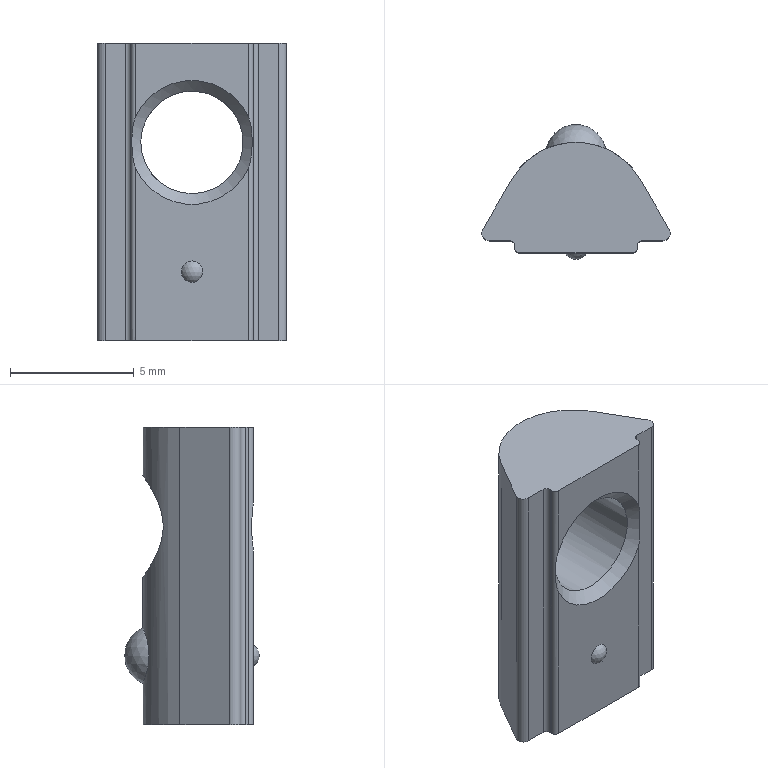Part | STEP file | 189654 HMBN-5-M5-189654 HMBN-5-M5 | 1 solid | 21 faces | box 7.6 x 5.445 x 12 mm | volume 233.461 mm3 | plane 10 | cylinder 8 | sphere 2 | cone 1 | commonest cylinder face diameters 0.4 x4 0.6 x2 4.134 x1 6 x1